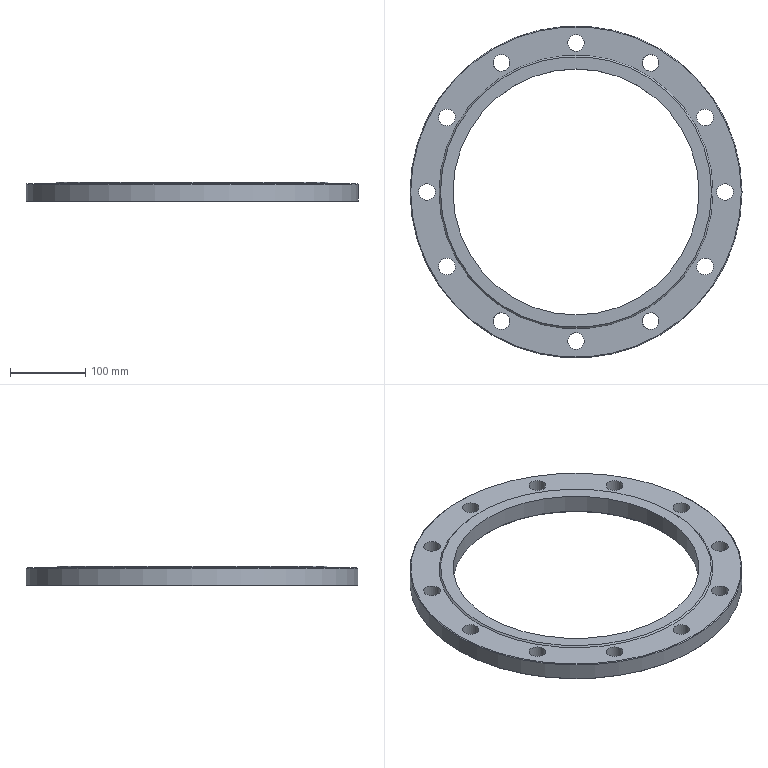Part | NX | features INSTANCE 12, ABSOLUTE_DATUM_PLANE 3, CHAMFER 3, SIMPLE HOLE 2, ABSOLUTE_DATUM_AXIS 1, BOSS 1, CIRCULAR_ISET 1, CYLINDER 1, TRANSFORM_ISET 1 | 1 solid | 21 faces | box 440 x 440 x 26 mm | volume 1570875 mm3 | cylinder 14 | cone 4 | plane 3 | commonest cylinder face diameters 22 x12 326 x1 440 x1
STEP:
#1=CARTESIAN_POINT('',(-180.566,104.25,24.));
#2=VERTEX_POINT('',#1);
#3=CARTESIAN_POINT('',(-171.04,98.75,24.));
#4=DIRECTION('',(0.,0.,-1.));
#5=DIRECTION('',(-0.866,0.5,0.));
#6=AXIS2_PLACEMENT_3D('',#3,#4,#5);
#7=CIRCLE('',#6,11.);
#8=EDGE_CURVE('',#2,#2,#7,.T.);
#9=ORIENTED_EDGE('',*,*,#8,.T.);
#10=EDGE_LOOP('',(#9));
#11=FACE_BOUND('',#10,.T.);
#12=CARTESIAN_POINT('',(-104.25,180.566,24.));
#13=VERTEX_POINT('',#12);
#14=CARTESIAN_POINT('',(-98.75,171.04,24.));
#15=DIRECTION('',(0.,0.,-1.));
#16=DIRECTION('',(-0.5,0.866,0.));
#17=AXIS2_PLACEMENT_3D('',#14,#15,#16);
#18=CIRCLE('',#17,11.);
#19=EDGE_CURVE('',#13,#13,#18,.T.);
#20=ORIENTED_EDGE('',*,*,#19,.T.);
#21=EDGE_LOOP('',(#20));
#22=FACE_BOUND('',#21,.T.);
#23=CARTESIAN_POINT('',(0.,208.5,24.));
#24=VERTEX_POINT('',#23);
#25=CARTESIAN_POINT('',(0.,197.5,24.));
#26=DIRECTION('',(0.,0.,-1.));
#27=DIRECTION('',(0.,1.,0.));
#28=AXIS2_PLACEMENT_3D('',#25,#26,#27);
#29=CIRCLE('',#28,11.);
#30=EDGE_CURVE('',#24,#24,#29,.T.);
#31=ORIENTED_EDGE('',*,*,#30,.T.);
#32=EDGE_LOOP('',(#31));
#33=FACE_BOUND('',#32,.T.);
#34=CARTESIAN_POINT('',(104.25,180.566,24.));
#35=VERTEX_POINT('',#34);
#36=CARTESIAN_POINT('',(98.75,171.04,24.));
#37=DIRECTION('',(0.,0.,-1.));
#38=DIRECTION('',(0.5,0.866,0.));
#39=AXIS2_PLACEMENT_3D('',#36,#37,#38);
#40=CIRCLE('',#39,11.);
#41=EDGE_CURVE('',#35,#35,#40,.T.);
#42=ORIENTED_EDGE('',*,*,#41,.T.);
#43=EDGE_LOOP('',(#42));
#44=FACE_BOUND('',#43,.T.);
#45=CARTESIAN_POINT('',(180.566,104.25,24.));
#46=VERTEX_POINT('',#45);
#47=CARTESIAN_POINT('',(171.04,98.75,24.));
#48=DIRECTION('',(0.,0.,-1.));
#49=DIRECTION('',(0.866,0.5,0.));
#50=AXIS2_PLACEMENT_3D('',#47,#48,#49);
#51=CIRCLE('',#50,11.);
#52=EDGE_CURVE('',#46,#46,#51,.T.);
#53=ORIENTED_EDGE('',*,*,#52,.T.);
#54=EDGE_LOOP('',(#53));
#55=FACE_BOUND('',#54,.T.);
#56=CARTESIAN_POINT('',(208.5,0.,24.));
#57=VERTEX_POINT('',#56);
#58=CARTESIAN_POINT('',(197.5,0.,24.));
#59=DIRECTION('',(0.,0.,-1.));
#60=DIRECTION('',(1.,0.,0.));
#61=AXIS2_PLACEMENT_3D('',#58,#59,#60);
#62=CIRCLE('',#61,11.);
#63=EDGE_CURVE('',#57,#57,#62,.T.);
#64=ORIENTED_EDGE('',*,*,#63,.T.);
#65=EDGE_LOOP('',(#64));
#66=FACE_BOUND('',#65,.T.);
#67=CARTESIAN_POINT('',(180.566,-104.25,24.));
#68=VERTEX_POINT('',#67);
#69=CARTESIAN_POINT('',(171.04,-98.75,24.));
#70=DIRECTION('',(0.,0.,-1.));
#71=DIRECTION('',(0.866,-0.5,0.));
#72=AXIS2_PLACEMENT_3D('',#69,#70,#71);
#73=CIRCLE('',#72,11.);
#74=EDGE_CURVE('',#68,#68,#73,.T.);
#75=ORIENTED_EDGE('',*,*,#74,.T.);
#76=EDGE_LOOP('',(#75));
#77=FACE_BOUND('',#76,.T.);
#78=CARTESIAN_POINT('',(104.25,-180.566,24.));
#79=VERTEX_POINT('',#78);
#80=CARTESIAN_POINT('',(98.75,-171.04,24.));
#81=DIRECTION('',(0.,0.,-1.));
#82=DIRECTION('',(0.5,-0.866,0.));
#83=AXIS2_PLACEMENT_3D('',#80,#81,#82);
#84=CIRCLE('',#83,11.);
#85=EDGE_CURVE('',#79,#79,#84,.T.);
#86=ORIENTED_EDGE('',*,*,#85,.T.);
#87=EDGE_LOOP('',(#86));
#88=FACE_BOUND('',#87,.T.);
#89=CARTESIAN_POINT('',(0.,-208.5,24.));
#90=VERTEX_POINT('',#89);
#91=CARTESIAN_POINT('',(0.,-197.5,24.));
#92=DIRECTION('',(0.,0.,-1.));
#93=DIRECTION('',(0.,-1.,0.));
#94=AXIS2_PLACEMENT_3D('',#91,#92,#93);
#95=CIRCLE('',#94,11.);
#96=EDGE_CURVE('',#90,#90,#95,.T.);
#97=ORIENTED_EDGE('',*,*,#96,.T.);
#98=EDGE_LOOP('',(#97));
#99=FACE_BOUND('',#98,.T.);
#100=CARTESIAN_POINT('',(-104.25,-180.566,24.));
#101=VERTEX_POINT('',#100);
#102=CARTESIAN_POINT('',(-98.75,-171.04,24.));
#103=DIRECTION('',(0.,0.,-1.));
#104=DIRECTION('',(-0.5,-0.866,0.));
#105=AXIS2_PLACEMENT_3D('',#102,#103,#104);
#106=CIRCLE('',#105,11.);
#107=EDGE_CURVE('',#101,#101,#106,.T.);
#108=ORIENTED_EDGE('',*,*,#107,.T.);
#109=EDGE_LOOP('',(#108));
#110=FACE_BOUND('',#109,.T.);
#111=CARTESIAN_POINT('',(-180.566,-104.25,24.));
#112=VERTEX_POINT('',#111);
#113=CARTESIAN_POINT('',(-171.04,-98.75,24.));
#114=DIRECTION('',(0.,0.,-1.));
#115=DIRECTION('',(-0.866,-0.5,0.));
#116=AXIS2_PLACEMENT_3D('',#113,#114,#115);
#117=CIRCLE('',#116,11.);
#118=EDGE_CURVE('',#112,#112,#117,.T.);
#119=ORIENTED_EDGE('',*,*,#118,.T.);
#120=EDGE_LOOP('',(#119));
#121=FACE_BOUND('',#120,.T.);
#122=CARTESIAN_POINT('',(-208.5,0.,24.));
#123=VERTEX_POINT('',#122);
#124=CARTESIAN_POINT('',(-197.5,0.,24.));
#125=DIRECTION('',(0.,0.,-1.));
#126=DIRECTION('',(-1.,0.,0.));
#127=AXIS2_PLACEMENT_3D('',#124,#125,#126);
#128=CIRCLE('',#127,11.);
#129=EDGE_CURVE('',#123,#123,#128,.T.);
#130=ORIENTED_EDGE('',*,*,#129,.T.);
#131=EDGE_LOOP('',(#130));
#132=FACE_BOUND('',#131,.T.);
#133=CARTESIAN_POINT('',(219.,0.,24.));
#134=VERTEX_POINT('',#133);
#135=CARTESIAN_POINT('',(0.,0.,24.));
#136=DIRECTION('',(0.,0.,1.));
#137=DIRECTION('',(1.,0.,0.));
#138=AXIS2_PLACEMENT_3D('',#135,#136,#137);
#139=CIRCLE('',#138,219.);
#140=EDGE_CURVE('',#134,#134,#139,.T.);
#141=ORIENTED_EDGE('',*,*,#140,.T.);
#142=EDGE_LOOP('',(#141));
#143=FACE_BOUND('',#142,.T.);
#144=CARTESIAN_POINT('',(181.5,0.,24.));
#145=VERTEX_POINT('',#144);
#146=CARTESIAN_POINT('',(0.,0.,24.));
#147=DIRECTION('',(0.,0.,1.));
#148=DIRECTION('',(1.,0.,0.));
#149=AXIS2_PLACEMENT_3D('',#146,#147,#148);
#150=CIRCLE('',#149,181.5);
#151=EDGE_CURVE('',#145,#145,#150,.T.);
#152=ORIENTED_EDGE('',*,*,#151,.F.);
#153=EDGE_LOOP('',(#152));
#154=FACE_BOUND('',#153,.T.);
#155=CARTESIAN_POINT('',(0.,0.,24.));
#156=DIRECTION('',(0.,0.,1.));
#157=DIRECTION('',(1.,0.,0.));
#158=AXIS2_PLACEMENT_3D('',#155,#156,#157);
#159=PLANE('',#158);
#160=ADVANCED_FACE('',(#11,#22,#33,#44,#55,#66,#77,#88,#99,#110,#121,#132,#143,#154),#159,.T.);
#161=CARTESIAN_POINT('',(-165.,0.,0.));
#162=VERTEX_POINT('',#161);
#163=CARTESIAN_POINT('',(0.,0.,0.));
#164=DIRECTION('',(0.,0.,-1.));
#165=DIRECTION('',(-1.,0.,0.));
#166=AXIS2_PLACEMENT_3D('',#163,#164,#165);
#167=CIRCLE('',#166,165.);
#168=EDGE_CURVE('',#162,#162,#167,.F.);
#169=ORIENTED_EDGE('',*,*,#168,.T.);
#170=EDGE_LOOP('',(#169));
#171=FACE_BOUND('',#170,.T.);
#172=CARTESIAN_POINT('',(-182.04,98.75,0.));
#173=VERTEX_POINT('',#172);
#174=CARTESIAN_POINT('',(-171.04,98.75,0.));
#175=DIRECTION('',(0.,0.,-1.));
#176=DIRECTION('',(-1.,0.,0.));
#177=AXIS2_PLACEMENT_3D('',#174,#175,#176);
#178=CIRCLE('',#177,11.);
#179=EDGE_CURVE('',#173,#173,#178,.T.);
#180=ORIENTED_EDGE('',*,*,#179,.F.);
#181=EDGE_LOOP('',(#180));
#182=FACE_BOUND('',#181,.T.);
#183=CARTESIAN_POINT('',(-109.75,171.04,0.));
#184=VERTEX_POINT('',#183);
#185=CARTESIAN_POINT('',(-98.75,171.04,0.));
#186=DIRECTION('',(0.,0.,-1.));
#187=DIRECTION('',(-1.,0.,0.));
#188=AXIS2_PLACEMENT_3D('',#185,#186,#187);
#189=CIRCLE('',#188,11.);
#190=EDGE_CURVE('',#184,#184,#189,.T.);
#191=ORIENTED_EDGE('',*,*,#190,.F.);
#192=EDGE_LOOP('',(#191));
#193=FACE_BOUND('',#192,.T.);
#194=CARTESIAN_POINT('',(-11.,197.5,0.));
#195=VERTEX_POINT('',#194);
#196=CARTESIAN_POINT('',(0.,197.5,0.));
#197=DIRECTION('',(0.,0.,-1.));
#198=DIRECTION('',(-1.,0.,0.));
#199=AXIS2_PLACEMENT_3D('',#196,#197,#198);
#200=CIRCLE('',#199,11.);
#201=EDGE_CURVE('',#195,#195,#200,.T.);
#202=ORIENTED_EDGE('',*,*,#201,.F.);
#203=EDGE_LOOP('',(#202));
#204=FACE_BOUND('',#203,.T.);
#205=CARTESIAN_POINT('',(87.75,171.04,0.));
#206=VERTEX_POINT('',#205);
#207=CARTESIAN_POINT('',(98.75,171.04,0.));
#208=DIRECTION('',(0.,0.,-1.));
#209=DIRECTION('',(-1.,0.,0.));
#210=AXIS2_PLACEMENT_3D('',#207,#208,#209);
#211=CIRCLE('',#210,11.);
#212=EDGE_CURVE('',#206,#206,#211,.T.);
#213=ORIENTED_EDGE('',*,*,#212,.F.);
#214=EDGE_LOOP('',(#213));
#215=FACE_BOUND('',#214,.T.);
#216=CARTESIAN_POINT('',(160.04,98.75,0.));
#217=VERTEX_POINT('',#216);
#218=CARTESIAN_POINT('',(171.04,98.75,0.));
#219=DIRECTION('',(0.,0.,-1.));
#220=DIRECTION('',(-1.,0.,0.));
#221=AXIS2_PLACEMENT_3D('',#218,#219,#220);
#222=CIRCLE('',#221,11.);
#223=EDGE_CURVE('',#217,#217,#222,.T.);
#224=ORIENTED_EDGE('',*,*,#223,.F.);
#225=EDGE_LOOP('',(#224));
#226=FACE_BOUND('',#225,.T.);
#227=CARTESIAN_POINT('',(186.5,0.,0.));
#228=VERTEX_POINT('',#227);
#229=CARTESIAN_POINT('',(197.5,0.,0.));
#230=DIRECTION('',(0.,0.,-1.));
#231=DIRECTION('',(-1.,0.,0.));
#232=AXIS2_PLACEMENT_3D('',#229,#230,#231);
#233=CIRCLE('',#232,11.);
#234=EDGE_CURVE('',#228,#228,#233,.T.);
#235=ORIENTED_EDGE('',*,*,#234,.F.);
#236=EDGE_LOOP('',(#235));
#237=FACE_BOUND('',#236,.T.);
#238=CARTESIAN_POINT('',(160.04,-98.75,0.));
#239=VERTEX_POINT('',#238);
#240=CARTESIAN_POINT('',(171.04,-98.75,0.));
#241=DIRECTION('',(0.,0.,-1.));
#242=DIRECTION('',(-1.,0.,0.));
#243=AXIS2_PLACEMENT_3D('',#240,#241,#242);
#244=CIRCLE('',#243,11.);
#245=EDGE_CURVE('',#239,#239,#244,.T.);
#246=ORIENTED_EDGE('',*,*,#245,.F.);
#247=EDGE_LOOP('',(#246));
#248=FACE_BOUND('',#247,.T.);
#249=CARTESIAN_POINT('',(87.75,-171.04,0.));
#250=VERTEX_POINT('',#249);
#251=CARTESIAN_POINT('',(98.75,-171.04,0.));
#252=DIRECTION('',(0.,0.,-1.));
#253=DIRECTION('',(-1.,0.,0.));
#254=AXIS2_PLACEMENT_3D('',#251,#252,#253);
#255=CIRCLE('',#254,11.);
#256=EDGE_CURVE('',#250,#250,#255,.T.);
#257=ORIENTED_EDGE('',*,*,#256,.F.);
#258=EDGE_LOOP('',(#257));
#259=FACE_BOUND('',#258,.T.);
#260=CARTESIAN_POINT('',(-11.,-197.5,0.));
#261=VERTEX_POINT('',#260);
#262=CARTESIAN_POINT('',(0.,-197.5,0.));
#263=DIRECTION('',(0.,0.,-1.));
#264=DIRECTION('',(-1.,0.,0.));
#265=AXIS2_PLACEMENT_3D('',#262,#263,#264);
#266=CIRCLE('',#265,11.);
#267=EDGE_CURVE('',#261,#261,#266,.T.);
#268=ORIENTED_EDGE('',*,*,#267,.F.);
#269=EDGE_LOOP('',(#268));
#270=FACE_BOUND('',#269,.T.);
#271=CARTESIAN_POINT('',(-109.75,-171.04,0.));
#272=VERTEX_POINT('',#271);
#273=CARTESIAN_POINT('',(-98.75,-171.04,0.));
#274=DIRECTION('',(0.,0.,-1.));
#275=DIRECTION('',(-1.,0.,0.));
#276=AXIS2_PLACEMENT_3D('',#273,#274,#275);
#277=CIRCLE('',#276,11.);
#278=EDGE_CURVE('',#272,#272,#277,.T.);
#279=ORIENTED_EDGE('',*,*,#278,.F.);
#280=EDGE_LOOP('',(#279));
#281=FACE_BOUND('',#280,.T.);
#282=CARTESIAN_POINT('',(-182.04,-98.75,0.));
#283=VERTEX_POINT('',#282);
#284=CARTESIAN_POINT('',(-171.04,-98.75,0.));
#285=DIRECTION('',(0.,0.,-1.));
#286=DIRECTION('',(-1.,0.,0.));
#287=AXIS2_PLACEMENT_3D('',#284,#285,#286);
#288=CIRCLE('',#287,11.);
#289=EDGE_CURVE('',#283,#283,#288,.T.);
#290=ORIENTED_EDGE('',*,*,#289,.F.);
#291=EDGE_LOOP('',(#290));
#292=FACE_BOUND('',#291,.T.);
#293=CARTESIAN_POINT('',(-208.5,0.,0.));
#294=VERTEX_POINT('',#293);
#295=CARTESIAN_POINT('',(-197.5,0.,0.));
#296=DIRECTION('',(0.,0.,-1.));
#297=DIRECTION('',(-1.,0.,0.));
#298=AXIS2_PLACEMENT_3D('',#295,#296,#297);
#299=CIRCLE('',#298,11.);
#300=EDGE_CURVE('',#294,#294,#299,.T.);
#301=ORIENTED_EDGE('',*,*,#300,.F.);
#302=EDGE_LOOP('',(#301));
#303=FACE_BOUND('',#302,.T.);
#304=CARTESIAN_POINT('',(-219.,0.,0.));
#305=VERTEX_POINT('',#304);
#306=CARTESIAN_POINT('',(0.,0.,0.));
#307=DIRECTION('',(0.,0.,-1.));
#308=DIRECTION('',(-1.,0.,0.));
#309=AXIS2_PLACEMENT_3D('',#306,#307,#308);
#310=CIRCLE('',#309,219.);
#311=EDGE_CURVE('',#305,#305,#310,.T.);
#312=ORIENTED_EDGE('',*,*,#311,.T.);
#313=EDGE_LOOP('',(#312));
#314=FACE_BOUND('',#313,.T.);
#315=CARTESIAN_POINT('',(0.,0.,0.));
#316=DIRECTION('',(0.,0.,-1.));
#317=DIRECTION('',(-1.,0.,0.));
#318=AXIS2_PLACEMENT_3D('',#315,#316,#317);
#319=PLANE('',#318);
#320=ADVANCED_FACE('',(#171,#182,#193,#204,#215,#226,#237,#248,#259,#270,#281,#292,#303,#314),#319,.T.);
#321=CARTESIAN_POINT('',(220.,0.,23.));
#322=VERTEX_POINT('',#321);
#323=CARTESIAN_POINT('',(0.,0.,23.));
#324=DIRECTION('',(0.,0.,1.));
#325=DIRECTION('',(1.,0.,0.));
#326=AXIS2_PLACEMENT_3D('',#323,#324,#325);
#327=CIRCLE('',#326,220.);
#328=EDGE_CURVE('',#322,#322,#327,.F.);
#329=ORIENTED_EDGE('',*,*,#328,.T.);
#330=EDGE_LOOP('',(#329));
#331=FACE_BOUND('',#330,.T.);
#332=CARTESIAN_POINT('',(-220.,0.,1.));
#333=VERTEX_POINT('',#332);
#334=CARTESIAN_POINT('',(0.,0.,1.));
#335=DIRECTION('',(0.,0.,-1.));
#336=DIRECTION('',(-1.,0.,0.));
#337=AXIS2_PLACEMENT_3D('',#334,#335,#336);
#338=CIRCLE('',#337,220.);
#339=EDGE_CURVE('',#333,#333,#338,.F.);
#340=ORIENTED_EDGE('',*,*,#339,.T.);
#341=EDGE_LOOP('',(#340));
#342=FACE_BOUND('',#341,.T.);
#343=CARTESIAN_POINT('',(0.,0.,0.));
#344=DIRECTION('',(0.,0.,1.));
#345=DIRECTION('',(1.,0.,0.));
#346=AXIS2_PLACEMENT_3D('',#343,#344,#345);
#347=CYLINDRICAL_SURFACE('',#346,220.);
#348=ADVANCED_FACE('',(#331,#342),#347,.T.);
#349=CARTESIAN_POINT('',(-163.,0.,26.));
#350=VERTEX_POINT('',#349);
#351=CARTESIAN_POINT('',(0.,0.,26.));
#352=DIRECTION('',(0.,0.,-1.));
#353=DIRECTION('',(-1.,0.,0.));
#354=AXIS2_PLACEMENT_3D('',#351,#352,#353);
#355=CIRCLE('',#354,163.);
#356=EDGE_CURVE('',#350,#350,#355,.T.);
#357=ORIENTED_EDGE('',*,*,#356,.T.);
#358=EDGE_LOOP('',(#357));
#359=FACE_BOUND('',#358,.T.);
#360=CARTESIAN_POINT('',(179.5,0.,26.));
#361=VERTEX_POINT('',#360);
#362=CARTESIAN_POINT('',(0.,0.,26.));
#363=DIRECTION('',(0.,0.,1.));
#364=DIRECTION('',(1.,0.,0.));
#365=AXIS2_PLACEMENT_3D('',#362,#363,#364);
#366=CIRCLE('',#365,179.5);
#367=EDGE_CURVE('',#361,#361,#366,.T.);
#368=ORIENTED_EDGE('',*,*,#367,.T.);
#369=EDGE_LOOP('',(#368));
#370=FACE_BOUND('',#369,.T.);
#371=CARTESIAN_POINT('',(0.,0.,26.));
#372=DIRECTION('',(0.,0.,1.));
#373=DIRECTION('',(1.,0.,0.));
#374=AXIS2_PLACEMENT_3D('',#371,#372,#373);
#375=PLANE('',#374);
#376=ADVANCED_FACE('',(#359,#370),#375,.T.);
#377=ORIENTED_EDGE('',*,*,#151,.T.);
#378=EDGE_LOOP('',(#377));
#379=FACE_BOUND('',#378,.T.);
#380=ORIENTED_EDGE('',*,*,#367,.F.);
#381=EDGE_LOOP('',(#380));
#382=FACE_BOUND('',#381,.T.);
#383=CARTESIAN_POINT('',(0.,0.,26.));
#384=DIRECTION('',(0.,0.,-1.));
#385=DIRECTION('',(-1.,0.,0.));
#386=AXIS2_PLACEMENT_3D('',#383,#384,#385);
#387=CONICAL_SURFACE('',#386,179.5,0.7854);
#388=ADVANCED_FACE('',(#379,#382),#387,.T.);
#389=ORIENTED_EDGE('',*,*,#140,.F.);
#390=EDGE_LOOP('',(#389));
#391=FACE_BOUND('',#390,.T.);
#392=ORIENTED_EDGE('',*,*,#328,.F.);
#393=EDGE_LOOP('',(#392));
#394=FACE_BOUND('',#393,.T.);
#395=CARTESIAN_POINT('',(0.,0.,23.));
#396=DIRECTION('',(0.,0.,-1.));
#397=DIRECTION('',(-1.,0.,0.));
#398=AXIS2_PLACEMENT_3D('',#395,#396,#397);
#399=CONICAL_SURFACE('',#398,220.,0.7854);
#400=ADVANCED_FACE('',(#391,#394),#399,.T.);
#401=ORIENTED_EDGE('',*,*,#311,.F.);
#402=EDGE_LOOP('',(#401));
#403=FACE_BOUND('',#402,.T.);
#404=ORIENTED_EDGE('',*,*,#339,.F.);
#405=EDGE_LOOP('',(#404));
#406=FACE_BOUND('',#405,.T.);
#407=CARTESIAN_POINT('',(0.,0.,1.));
#408=DIRECTION('',(0.,0.,1.));
#409=DIRECTION('',(1.,0.,0.));
#410=AXIS2_PLACEMENT_3D('',#407,#408,#409);
#411=CONICAL_SURFACE('',#410,220.,0.7854);
#412=ADVANCED_FACE('',(#403,#406),#411,.T.);
#413=ORIENTED_EDGE('',*,*,#300,.T.);
#414=EDGE_LOOP('',(#413));
#415=FACE_BOUND('',#414,.T.);
#416=ORIENTED_EDGE('',*,*,#129,.F.);
#417=EDGE_LOOP('',(#416));
#418=FACE_BOUND('',#417,.T.);
#419=CARTESIAN_POINT('',(-197.5,0.,24.));
#420=DIRECTION('',(0.,0.,-1.));
#421=DIRECTION('',(-1.,0.,0.));
#422=AXIS2_PLACEMENT_3D('',#419,#420,#421);
#423=CYLINDRICAL_SURFACE('',#422,11.);
#424=ADVANCED_FACE('',(#415,#418),#423,.F.);
#425=CARTESIAN_POINT('',(-163.,0.,2.));
#426=VERTEX_POINT('',#425);
#427=CARTESIAN_POINT('',(0.,0.,2.));
#428=DIRECTION('',(0.,0.,-1.));
#429=DIRECTION('',(-1.,0.,0.));
#430=AXIS2_PLACEMENT_3D('',#427,#428,#429);
#431=CIRCLE('',#430,163.);
#432=EDGE_CURVE('',#426,#426,#431,.T.);
#433=ORIENTED_EDGE('',*,*,#432,.T.);
#434=EDGE_LOOP('',(#433));
#435=FACE_BOUND('',#434,.T.);
#436=ORIENTED_EDGE('',*,*,#356,.F.);
#437=EDGE_LOOP('',(#436));
#438=FACE_BOUND('',#437,.T.);
#439=CARTESIAN_POINT('',(0.,0.,26.));
#440=DIRECTION('',(0.,0.,-1.));
#441=DIRECTION('',(-1.,0.,0.));
#442=AXIS2_PLACEMENT_3D('',#439,#440,#441);
#443=CYLINDRICAL_SURFACE('',#442,163.);
#444=ADVANCED_FACE('',(#435,#438),#443,.F.);
#445=ORIENTED_EDGE('',*,*,#289,.T.);
#446=EDGE_LOOP('',(#445));
#447=FACE_BOUND('',#446,.T.);
#448=ORIENTED_EDGE('',*,*,#118,.F.);
#449=EDGE_LOOP('',(#448));
#450=FACE_BOUND('',#449,.T.);
#451=CARTESIAN_POINT('',(-171.04,-98.75,24.));
#452=DIRECTION('',(0.,0.,-1.));
#453=DIRECTION('',(-0.866,-0.5,0.));
#454=AXIS2_PLACEMENT_3D('',#451,#452,#453);
#455=CYLINDRICAL_SURFACE('',#454,11.);
#456=ADVANCED_FACE('',(#447,#450),#455,.F.);
#457=ORIENTED_EDGE('',*,*,#278,.T.);
#458=EDGE_LOOP('',(#457));
#459=FACE_BOUND('',#458,.T.);
#460=ORIENTED_EDGE('',*,*,#107,.F.);
#461=EDGE_LOOP('',(#460));
#462=FACE_BOUND('',#461,.T.);
#463=CARTESIAN_POINT('',(-98.75,-171.04,24.));
#464=DIRECTION('',(0.,0.,-1.));
#465=DIRECTION('',(-0.5,-0.866,0.));
#466=AXIS2_PLACEMENT_3D('',#463,#464,#465);
#467=CYLINDRICAL_SURFACE('',#466,11.);
#468=ADVANCED_FACE('',(#459,#462),#467,.F.);
#469=ORIENTED_EDGE('',*,*,#267,.T.);
#470=EDGE_LOOP('',(#469));
#471=FACE_BOUND('',#470,.T.);
#472=ORIENTED_EDGE('',*,*,#96,.F.);
#473=EDGE_LOOP('',(#472));
#474=FACE_BOUND('',#473,.T.);
#475=CARTESIAN_POINT('',(0.,-197.5,24.));
#476=DIRECTION('',(0.,0.,-1.));
#477=DIRECTION('',(0.,-1.,0.));
#478=AXIS2_PLACEMENT_3D('',#475,#476,#477);
#479=CYLINDRICAL_SURFACE('',#478,11.);
#480=ADVANCED_FACE('',(#471,#474),#479,.F.);
#481=ORIENTED_EDGE('',*,*,#256,.T.);
#482=EDGE_LOOP('',(#481));
#483=FACE_BOUND('',#482,.T.);
#484=ORIENTED_EDGE('',*,*,#85,.F.);
#485=EDGE_LOOP('',(#484));
#486=FACE_BOUND('',#485,.T.);
#487=CARTESIAN_POINT('',(98.75,-171.04,24.));
#488=DIRECTION('',(0.,0.,-1.));
#489=DIRECTION('',(0.5,-0.866,0.));
#490=AXIS2_PLACEMENT_3D('',#487,#488,#489);
#491=CYLINDRICAL_SURFACE('',#490,11.);
#492=ADVANCED_FACE('',(#483,#486),#491,.F.);
#493=ORIENTED_EDGE('',*,*,#245,.T.);
#494=EDGE_LOOP('',(#493));
#495=FACE_BOUND('',#494,.T.);
#496=ORIENTED_EDGE('',*,*,#74,.F.);
#497=EDGE_LOOP('',(#496));
#498=FACE_BOUND('',#497,.T.);
#499=CARTESIAN_POINT('',(171.04,-98.75,24.));
#500=DIRECTION('',(0.,0.,-1.));
#501=DIRECTION('',(0.866,-0.5,0.));
#502=AXIS2_PLACEMENT_3D('',#499,#500,#501);
#503=CYLINDRICAL_SURFACE('',#502,11.);
#504=ADVANCED_FACE('',(#495,#498),#503,.F.);
#505=ORIENTED_EDGE('',*,*,#234,.T.);
#506=EDGE_LOOP('',(#505));
#507=FACE_BOUND('',#506,.T.);
#508=ORIENTED_EDGE('',*,*,#63,.F.);
#509=EDGE_LOOP('',(#508));
#510=FACE_BOUND('',#509,.T.);
#511=CARTESIAN_POINT('',(197.5,0.,24.));
#512=DIRECTION('',(0.,0.,-1.));
#513=DIRECTION('',(1.,0.,0.));
#514=AXIS2_PLACEMENT_3D('',#511,#512,#513);
#515=CYLINDRICAL_SURFACE('',#514,11.);
#516=ADVANCED_FACE('',(#507,#510),#515,.F.);
#517=ORIENTED_EDGE('',*,*,#223,.T.);
#518=EDGE_LOOP('',(#517));
#519=FACE_BOUND('',#518,.T.);
#520=ORIENTED_EDGE('',*,*,#52,.F.);
#521=EDGE_LOOP('',(#520));
#522=FACE_BOUND('',#521,.T.);
#523=CARTESIAN_POINT('',(171.04,98.75,24.));
#524=DIRECTION('',(0.,0.,-1.));
#525=DIRECTION('',(0.866,0.5,0.));
#526=AXIS2_PLACEMENT_3D('',#523,#524,#525);
#527=CYLINDRICAL_SURFACE('',#526,11.);
#528=ADVANCED_FACE('',(#519,#522),#527,.F.);
#529=ORIENTED_EDGE('',*,*,#212,.T.);
#530=EDGE_LOOP('',(#529));
#531=FACE_BOUND('',#530,.T.);
#532=ORIENTED_EDGE('',*,*,#41,.F.);
#533=EDGE_LOOP('',(#532));
#534=FACE_BOUND('',#533,.T.);
#535=CARTESIAN_POINT('',(98.75,171.04,24.));
#536=DIRECTION('',(0.,0.,-1.));
#537=DIRECTION('',(0.5,0.866,0.));
#538=AXIS2_PLACEMENT_3D('',#535,#536,#537);
#539=CYLINDRICAL_SURFACE('',#538,11.);
#540=ADVANCED_FACE('',(#531,#534),#539,.F.);
#541=ORIENTED_EDGE('',*,*,#201,.T.);
#542=EDGE_LOOP('',(#541));
#543=FACE_BOUND('',#542,.T.);
#544=ORIENTED_EDGE('',*,*,#30,.F.);
#545=EDGE_LOOP('',(#544));
#546=FACE_BOUND('',#545,.T.);
#547=CARTESIAN_POINT('',(0.,197.5,24.));
#548=DIRECTION('',(0.,0.,-1.));
#549=DIRECTION('',(0.,1.,0.));
#550=AXIS2_PLACEMENT_3D('',#547,#548,#549);
#551=CYLINDRICAL_SURFACE('',#550,11.);
#552=ADVANCED_FACE('',(#543,#546),#551,.F.);
#553=ORIENTED_EDGE('',*,*,#190,.T.);
#554=EDGE_LOOP('',(#553));
#555=FACE_BOUND('',#554,.T.);
#556=ORIENTED_EDGE('',*,*,#19,.F.);
#557=EDGE_LOOP('',(#556));
#558=FACE_BOUND('',#557,.T.);
#559=CARTESIAN_POINT('',(-98.75,171.04,24.));
#560=DIRECTION('',(0.,0.,-1.));
#561=DIRECTION('',(-0.5,0.866,0.));
#562=AXIS2_PLACEMENT_3D('',#559,#560,#561);
#563=CYLINDRICAL_SURFACE('',#562,11.);
#564=ADVANCED_FACE('',(#555,#558),#563,.F.);
#565=ORIENTED_EDGE('',*,*,#179,.T.);
#566=EDGE_LOOP('',(#565));
#567=FACE_BOUND('',#566,.T.);
#568=ORIENTED_EDGE('',*,*,#8,.F.);
#569=EDGE_LOOP('',(#568));
#570=FACE_BOUND('',#569,.T.);
#571=CARTESIAN_POINT('',(-171.04,98.75,24.));
#572=DIRECTION('',(0.,0.,-1.));
#573=DIRECTION('',(-0.866,0.5,0.));
#574=AXIS2_PLACEMENT_3D('',#571,#572,#573);
#575=CYLINDRICAL_SURFACE('',#574,11.);
#576=ADVANCED_FACE('',(#567,#570),#575,.F.);
#577=ORIENTED_EDGE('',*,*,#168,.F.);
#578=EDGE_LOOP('',(#577));
#579=FACE_BOUND('',#578,.T.);
#580=ORIENTED_EDGE('',*,*,#432,.F.);
#581=EDGE_LOOP('',(#580));
#582=FACE_BOUND('',#581,.T.);
#583=CARTESIAN_POINT('',(0.,0.,2.));
#584=DIRECTION('',(0.,0.,-1.));
#585=DIRECTION('',(-1.,0.,0.));
#586=AXIS2_PLACEMENT_3D('',#583,#584,#585);
#587=CONICAL_SURFACE('',#586,163.,0.7854);
#588=ADVANCED_FACE('',(#579,#582),#587,.F.);
#589=CLOSED_SHELL('',(#160,#320,#348,#376,#388,#400,#412,#424,#444,#456,#468,#480,#492,#504,#516,#528,#540,#552,#564,#576,#588));
#590=MANIFOLD_SOLID_BREP('',#589);
#591=(LENGTH_UNIT()NAMED_UNIT(*)SI_UNIT(.MILLI.,.METRE.));
#592=UNCERTAINTY_MEASURE_WITH_UNIT(LENGTH_MEASURE(0.00001),#591,'','');
#593=(NAMED_UNIT(*)PLANE_ANGLE_UNIT()SI_UNIT($,.RADIAN.));
#594=(NAMED_UNIT(*)SI_UNIT($,.STERADIAN.)SOLID_ANGLE_UNIT());
#595=(GEOMETRIC_REPRESENTATION_CONTEXT(3)GLOBAL_UNCERTAINTY_ASSIGNED_CONTEXT((#592))GLOBAL_UNIT_ASSIGNED_CONTEXT((#591,#593,#594))REPRESENTATION_CONTEXT('',''));
#596=ADVANCED_BREP_SHAPE_REPRESENTATION('',(#590),#595);